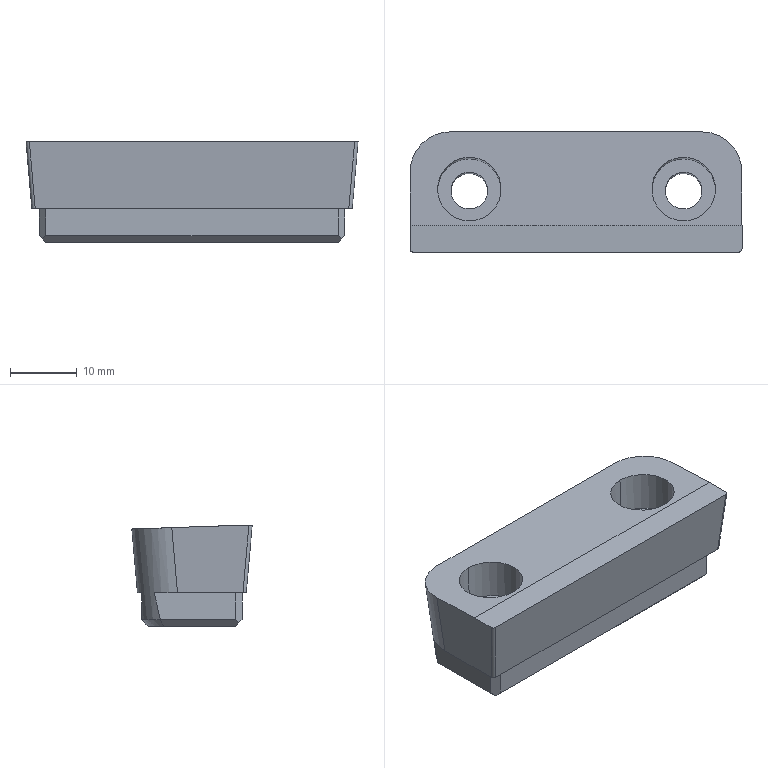Part | Creo | 1 solid | 47 faces | box 49.562 x 17.957 x 15 mm | volume 9919 mm3 | plane 25 | cylinder 16 | cone 4 | spline 2 | commonest cylinder face diameters 5.5 x4 8 x4 9.5 x4 1 x2 12 x2